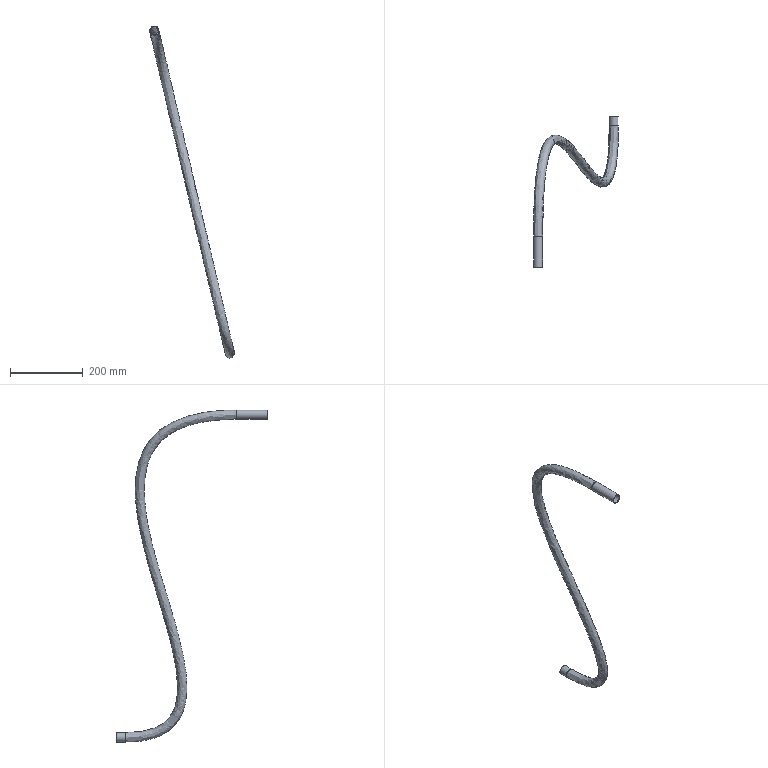Part | STEP file | Part 2^JBJ-F-0000-00 | 1 solid | 8 faces | box 234.291 x 415.992 x 914.606 mm | volume 198661 mm3 | cylinder 4 | spline 2 | plane 2 | commonest cylinder face diameters 22 x2 26 x2